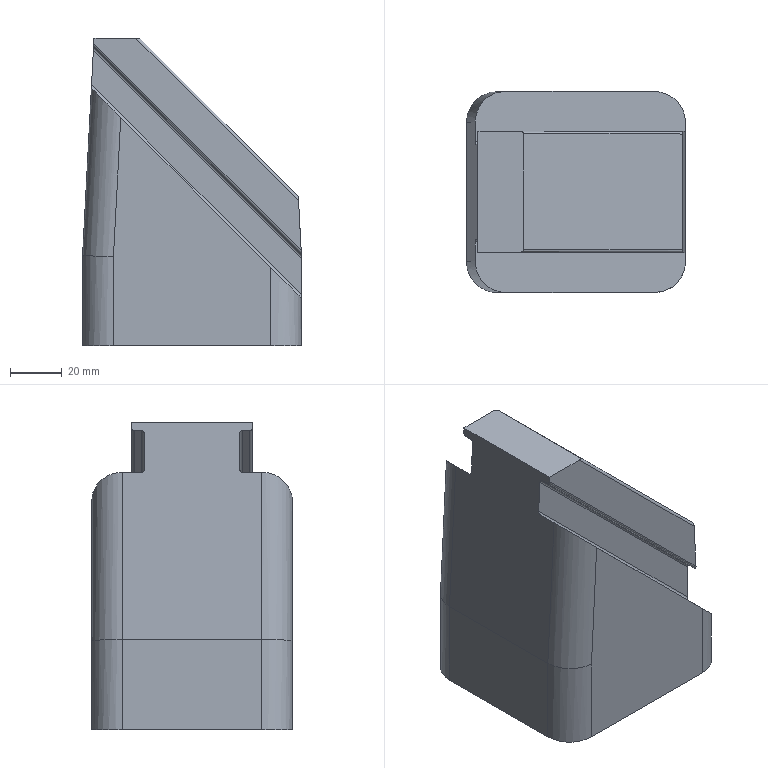Part | STEP file | solid 137 | 1 solid | 47 faces | box 85 x 78 x 119.504 mm | volume 501919 mm3 | cylinder 22 | plane 21 | cone 4 | commonest cylinder face diameters 2 x8 24 x6 10.2 x4 12 x4